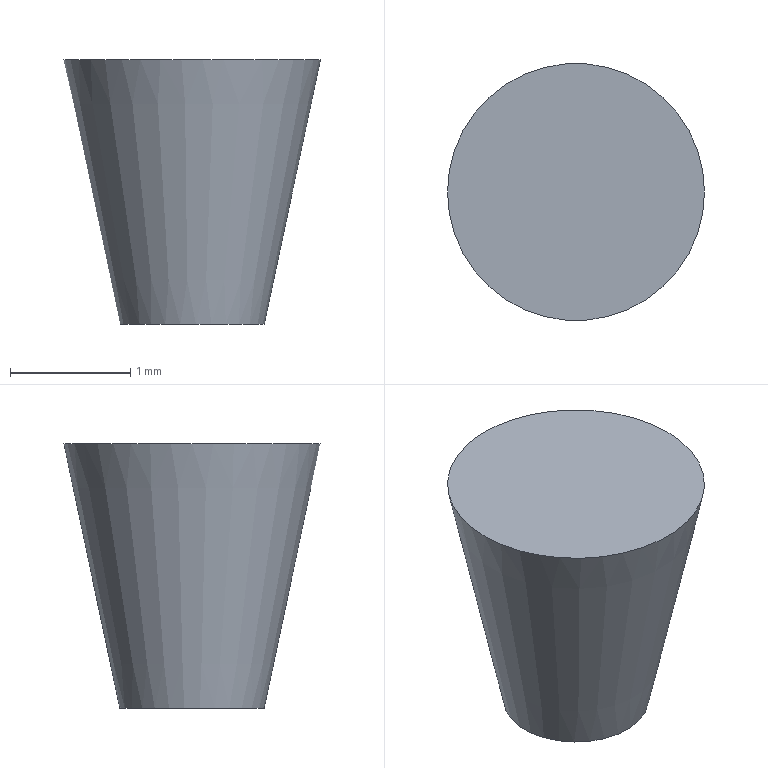Part | NX | features solid 2 | 1 solid | 3 faces | box 2.135 x 2.135 x 2.2 mm | volume 4.931 mm3 | plane 2 | cone 1
STEP:
#1=CARTESIAN_POINT('',(0.6,0.,22.04));
#2=VERTEX_POINT('',#1);
#3=CARTESIAN_POINT('',(0.,0.,22.04));
#4=DIRECTION('',(0.,0.,1.));
#5=DIRECTION('',(1.,0.,0.));
#6=AXIS2_PLACEMENT_3D('',#3,#4,#5);
#7=CIRCLE('',#6,0.6);
#8=EDGE_CURVE('',#2,#2,#7,.T.);
#9=ORIENTED_EDGE('',*,*,#8,.F.);
#10=EDGE_LOOP('',(#9));
#11=FACE_BOUND('',#10,.T.);
#12=CARTESIAN_POINT('',(0.,0.,22.04));
#13=DIRECTION('',(0.,0.,-1.));
#14=DIRECTION('',(-1.,0.,0.));
#15=AXIS2_PLACEMENT_3D('',#12,#13,#14);
#16=PLANE('',#15);
#17=ADVANCED_FACE('',(#11),#16,.T.);
#18=CARTESIAN_POINT('',(1.068,0.,24.24));
#19=VERTEX_POINT('',#18);
#20=CARTESIAN_POINT('',(0.,0.,24.24));
#21=DIRECTION('',(0.,0.,-1.));
#22=DIRECTION('',(1.,0.,0.));
#23=AXIS2_PLACEMENT_3D('',#20,#21,#22);
#24=CIRCLE('',#23,1.068);
#25=EDGE_CURVE('',#19,#19,#24,.T.);
#26=ORIENTED_EDGE('',*,*,#25,.F.);
#27=EDGE_LOOP('',(#26));
#28=FACE_BOUND('',#27,.T.);
#29=CARTESIAN_POINT('',(0.,0.,24.24));
#30=DIRECTION('',(0.,0.,1.));
#31=DIRECTION('',(1.,0.,0.));
#32=AXIS2_PLACEMENT_3D('',#29,#30,#31);
#33=PLANE('',#32);
#34=ADVANCED_FACE('',(#28),#33,.T.);
#35=ORIENTED_EDGE('',*,*,#8,.T.);
#36=EDGE_LOOP('',(#35));
#37=FACE_BOUND('',#36,.T.);
#38=ORIENTED_EDGE('',*,*,#25,.T.);
#39=EDGE_LOOP('',(#38));
#40=FACE_BOUND('',#39,.T.);
#41=CARTESIAN_POINT('',(0.,0.,22.04));
#42=DIRECTION('',(0.,0.,1.));
#43=DIRECTION('',(1.,0.,0.));
#44=AXIS2_PLACEMENT_3D('',#41,#42,#43);
#45=CONICAL_SURFACE('',#44,0.6,0.2094);
#46=ADVANCED_FACE('',(#37,#40),#45,.T.);
#47=CLOSED_SHELL('',(#17,#34,#46));
#48=MANIFOLD_SOLID_BREP('',#47);
#49=(LENGTH_UNIT()NAMED_UNIT(*)SI_UNIT(.MILLI.,.METRE.));
#50=UNCERTAINTY_MEASURE_WITH_UNIT(LENGTH_MEASURE(0.00001),#49,'','');
#51=(NAMED_UNIT(*)PLANE_ANGLE_UNIT()SI_UNIT($,.RADIAN.));
#52=(NAMED_UNIT(*)SI_UNIT($,.STERADIAN.)SOLID_ANGLE_UNIT());
#53=(GEOMETRIC_REPRESENTATION_CONTEXT(3)GLOBAL_UNCERTAINTY_ASSIGNED_CONTEXT((#50))GLOBAL_UNIT_ASSIGNED_CONTEXT((#49,#51,#52))REPRESENTATION_CONTEXT('',''));
#54=ADVANCED_BREP_SHAPE_REPRESENTATION('',(#48),#53);